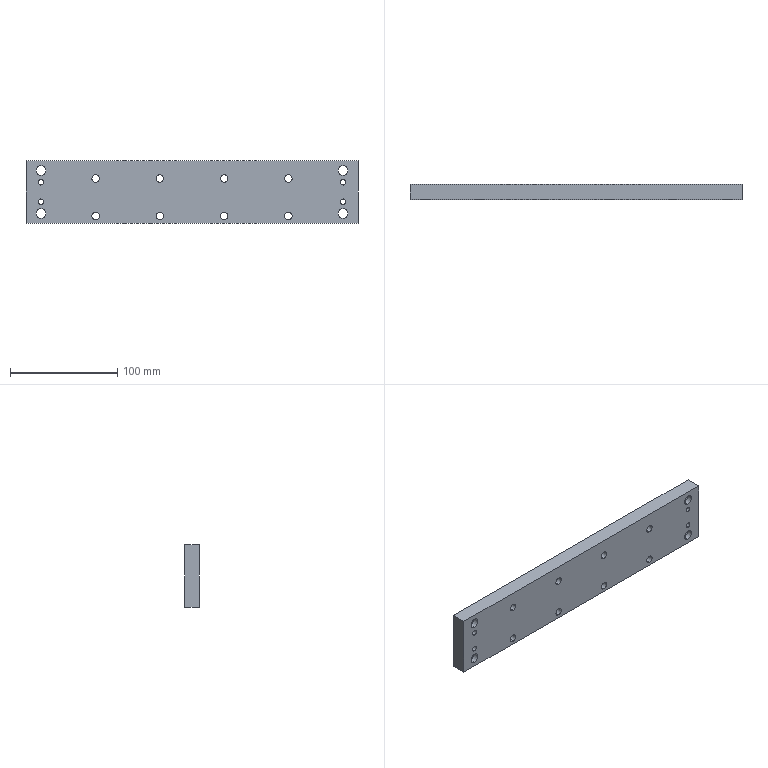Part | STEP file | PN_0023 base plate | 1 solid | 50 faces | box 310 x 14 x 58 mm | volume 238676 mm3 | cylinder 40 | plane 10 | commonest cylinder face diameters 7 x16 5 x8 9 x8 15 x8